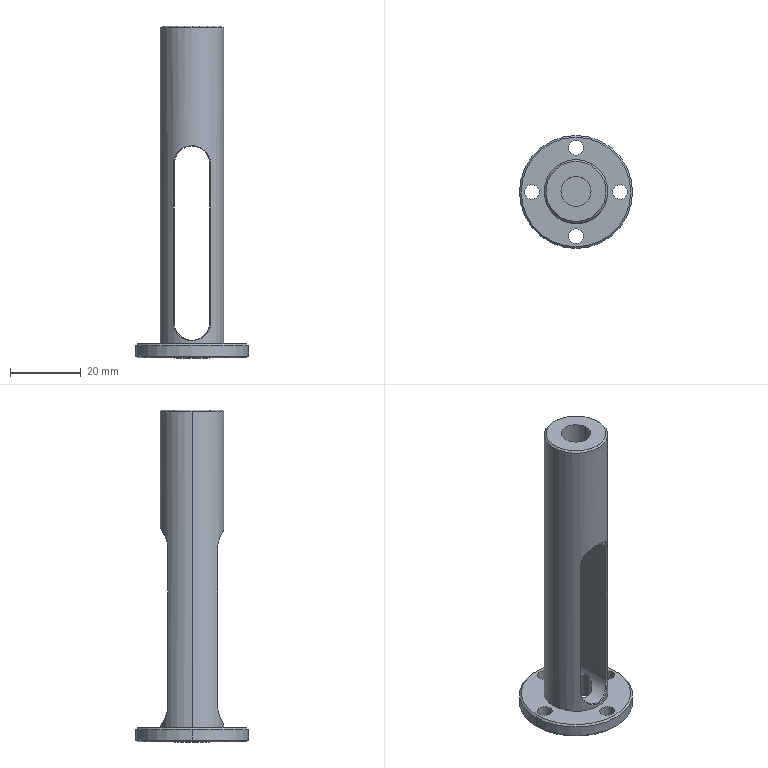Part | STEP file | Handle rod | 1 solid | 41 faces | box 32 x 32 x 94 mm | volume 15016 mm3 | cylinder 19 | plane 10 | cone 8 | spline 4 | commonest cylinder face diameters 4.2 x8 10 x3 8.5 x2 9 x2 18 x2 32 x2